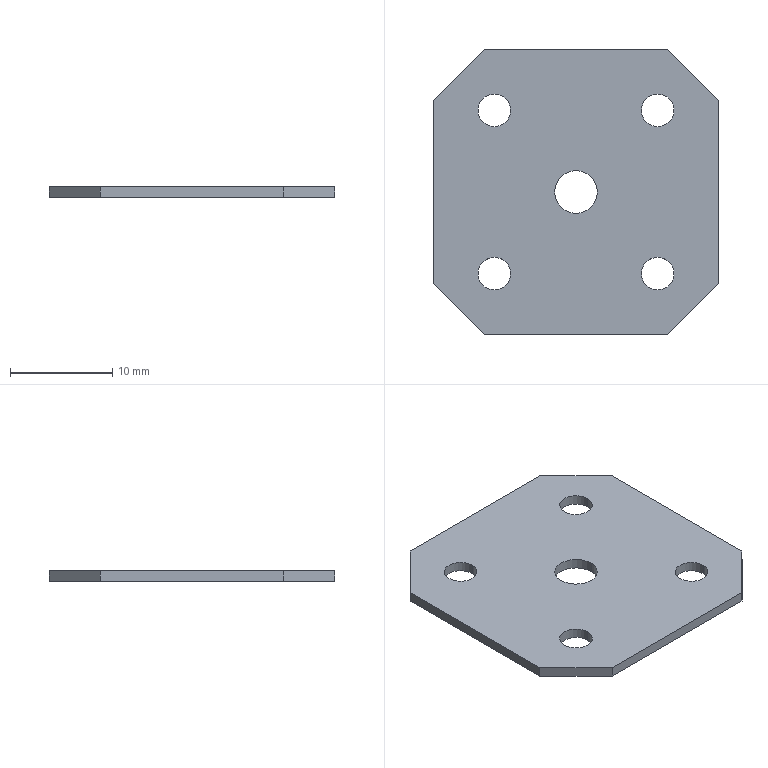Part | SolidWorks | features BaseBody 1 | 1 solid | 20 faces | box 28 x 28 x 1 mm | volume 688.173 mm3 | cylinder 10 | plane 10 | commonest cylinder face diameters 3.2 x8 4.17 x2
STEP:
#1=CARTESIAN_POINT('',(-2.085,0.,1.));
#2=VERTEX_POINT('',#1);
#3=CARTESIAN_POINT('',(2.085,0.,1.));
#4=VERTEX_POINT('',#3);
#5=CARTESIAN_POINT('',(0.,0.,1.));
#6=DIRECTION('',(0.,0.,1.));
#7=DIRECTION('',(-1.,0.,0.));
#8=AXIS2_PLACEMENT_3D('',#5,#6,#7);
#9=CIRCLE('',#8,2.085);
#10=EDGE_CURVE('',#2,#4,#9,.T.);
#11=ORIENTED_EDGE('',*,*,#10,.T.);
#12=CARTESIAN_POINT('',(2.085,0.,0.));
#13=VERTEX_POINT('',#12);
#14=CARTESIAN_POINT('',(2.085,0.,1.));
#15=DIRECTION('',(0.,0.,-1.));
#16=VECTOR('',#15,1000.);
#17=LINE('',#14,#16);
#18=EDGE_CURVE('',#4,#13,#17,.T.);
#19=ORIENTED_EDGE('',*,*,#18,.T.);
#20=CARTESIAN_POINT('',(-2.085,0.,0.));
#21=VERTEX_POINT('',#20);
#22=CARTESIAN_POINT('',(0.,0.,0.));
#23=DIRECTION('',(0.,0.,-1.));
#24=DIRECTION('',(-1.,0.,0.));
#25=AXIS2_PLACEMENT_3D('',#22,#23,#24);
#26=CIRCLE('',#25,2.085);
#27=EDGE_CURVE('',#13,#21,#26,.T.);
#28=ORIENTED_EDGE('',*,*,#27,.T.);
#29=CARTESIAN_POINT('',(-2.085,0.,1.));
#30=DIRECTION('',(0.,0.,-1.));
#31=VECTOR('',#30,1000.);
#32=LINE('',#29,#31);
#33=EDGE_CURVE('',#2,#21,#32,.T.);
#34=ORIENTED_EDGE('',*,*,#33,.F.);
#35=EDGE_LOOP('',(#11,#19,#28,#34));
#36=FACE_OUTER_BOUND('',#35,.T.);
#37=CARTESIAN_POINT('',(0.,0.,1.));
#38=DIRECTION('',(0.,0.,-1.));
#39=DIRECTION('',(-1.,0.,0.));
#40=AXIS2_PLACEMENT_3D('',#37,#38,#39);
#41=CYLINDRICAL_SURFACE('',#40,2.085);
#42=ADVANCED_FACE('',(#36),#41,.F.);
#43=CARTESIAN_POINT('',(9.6,-8.,1.));
#44=VERTEX_POINT('',#43);
#45=CARTESIAN_POINT('',(6.4,-8.,1.));
#46=VERTEX_POINT('',#45);
#47=CARTESIAN_POINT('',(8.,-8.,1.));
#48=DIRECTION('',(0.,0.,-1.));
#49=DIRECTION('',(-1.,0.,0.));
#50=AXIS2_PLACEMENT_3D('',#47,#48,#49);
#51=CIRCLE('',#50,1.6);
#52=EDGE_CURVE('',#44,#46,#51,.T.);
#53=ORIENTED_EDGE('',*,*,#52,.F.);
#54=CARTESIAN_POINT('',(9.6,-8.,0.));
#55=VERTEX_POINT('',#54);
#56=CARTESIAN_POINT('',(9.6,-8.,1.));
#57=DIRECTION('',(0.,0.,-1.));
#58=VECTOR('',#57,1000.);
#59=LINE('',#56,#58);
#60=EDGE_CURVE('',#44,#55,#59,.T.);
#61=ORIENTED_EDGE('',*,*,#60,.T.);
#62=CARTESIAN_POINT('',(6.4,-8.,0.));
#63=VERTEX_POINT('',#62);
#64=CARTESIAN_POINT('',(8.,-8.,0.));
#65=DIRECTION('',(0.,0.,-1.));
#66=DIRECTION('',(-1.,0.,0.));
#67=AXIS2_PLACEMENT_3D('',#64,#65,#66);
#68=CIRCLE('',#67,1.6);
#69=EDGE_CURVE('',#55,#63,#68,.T.);
#70=ORIENTED_EDGE('',*,*,#69,.T.);
#71=CARTESIAN_POINT('',(6.4,-8.,1.));
#72=DIRECTION('',(0.,0.,-1.));
#73=VECTOR('',#72,1000.);
#74=LINE('',#71,#73);
#75=EDGE_CURVE('',#46,#63,#74,.T.);
#76=ORIENTED_EDGE('',*,*,#75,.F.);
#77=EDGE_LOOP('',(#53,#61,#70,#76));
#78=FACE_OUTER_BOUND('',#77,.T.);
#79=CARTESIAN_POINT('',(8.,-8.,1.));
#80=DIRECTION('',(0.,0.,-1.));
#81=DIRECTION('',(-1.,0.,0.));
#82=AXIS2_PLACEMENT_3D('',#79,#80,#81);
#83=CYLINDRICAL_SURFACE('',#82,1.6);
#84=ADVANCED_FACE('',(#78),#83,.F.);
#85=CARTESIAN_POINT('',(-6.4,8.,1.));
#86=VERTEX_POINT('',#85);
#87=CARTESIAN_POINT('',(-9.6,8.,1.));
#88=VERTEX_POINT('',#87);
#89=CARTESIAN_POINT('',(-8.,8.,1.));
#90=DIRECTION('',(0.,0.,-1.));
#91=DIRECTION('',(-1.,0.,0.));
#92=AXIS2_PLACEMENT_3D('',#89,#90,#91);
#93=CIRCLE('',#92,1.6);
#94=EDGE_CURVE('',#86,#88,#93,.T.);
#95=ORIENTED_EDGE('',*,*,#94,.F.);
#96=CARTESIAN_POINT('',(-6.4,8.,0.));
#97=VERTEX_POINT('',#96);
#98=CARTESIAN_POINT('',(-6.4,8.,1.));
#99=DIRECTION('',(0.,0.,-1.));
#100=VECTOR('',#99,1000.);
#101=LINE('',#98,#100);
#102=EDGE_CURVE('',#86,#97,#101,.T.);
#103=ORIENTED_EDGE('',*,*,#102,.T.);
#104=CARTESIAN_POINT('',(-9.6,8.,0.));
#105=VERTEX_POINT('',#104);
#106=CARTESIAN_POINT('',(-8.,8.,0.));
#107=DIRECTION('',(0.,0.,-1.));
#108=DIRECTION('',(-1.,0.,0.));
#109=AXIS2_PLACEMENT_3D('',#106,#107,#108);
#110=CIRCLE('',#109,1.6);
#111=EDGE_CURVE('',#97,#105,#110,.T.);
#112=ORIENTED_EDGE('',*,*,#111,.T.);
#113=CARTESIAN_POINT('',(-9.6,8.,1.));
#114=DIRECTION('',(0.,0.,-1.));
#115=VECTOR('',#114,1000.);
#116=LINE('',#113,#115);
#117=EDGE_CURVE('',#88,#105,#116,.T.);
#118=ORIENTED_EDGE('',*,*,#117,.F.);
#119=EDGE_LOOP('',(#95,#103,#112,#118));
#120=FACE_OUTER_BOUND('',#119,.T.);
#121=CARTESIAN_POINT('',(-8.,8.,1.));
#122=DIRECTION('',(0.,0.,-1.));
#123=DIRECTION('',(-1.,0.,0.));
#124=AXIS2_PLACEMENT_3D('',#121,#122,#123);
#125=CYLINDRICAL_SURFACE('',#124,1.6);
#126=ADVANCED_FACE('',(#120),#125,.F.);
#127=CARTESIAN_POINT('',(9.6,8.,1.));
#128=VERTEX_POINT('',#127);
#129=CARTESIAN_POINT('',(6.4,8.,1.));
#130=VERTEX_POINT('',#129);
#131=CARTESIAN_POINT('',(8.,8.,1.));
#132=DIRECTION('',(0.,0.,-1.));
#133=DIRECTION('',(-1.,0.,0.));
#134=AXIS2_PLACEMENT_3D('',#131,#132,#133);
#135=CIRCLE('',#134,1.6);
#136=EDGE_CURVE('',#128,#130,#135,.T.);
#137=ORIENTED_EDGE('',*,*,#136,.F.);
#138=CARTESIAN_POINT('',(9.6,8.,0.));
#139=VERTEX_POINT('',#138);
#140=CARTESIAN_POINT('',(9.6,8.,1.));
#141=DIRECTION('',(0.,0.,-1.));
#142=VECTOR('',#141,1000.);
#143=LINE('',#140,#142);
#144=EDGE_CURVE('',#128,#139,#143,.T.);
#145=ORIENTED_EDGE('',*,*,#144,.T.);
#146=CARTESIAN_POINT('',(6.4,8.,0.));
#147=VERTEX_POINT('',#146);
#148=CARTESIAN_POINT('',(8.,8.,0.));
#149=DIRECTION('',(0.,0.,-1.));
#150=DIRECTION('',(-1.,0.,0.));
#151=AXIS2_PLACEMENT_3D('',#148,#149,#150);
#152=CIRCLE('',#151,1.6);
#153=EDGE_CURVE('',#139,#147,#152,.T.);
#154=ORIENTED_EDGE('',*,*,#153,.T.);
#155=CARTESIAN_POINT('',(6.4,8.,1.));
#156=DIRECTION('',(0.,0.,-1.));
#157=VECTOR('',#156,1000.);
#158=LINE('',#155,#157);
#159=EDGE_CURVE('',#130,#147,#158,.T.);
#160=ORIENTED_EDGE('',*,*,#159,.F.);
#161=EDGE_LOOP('',(#137,#145,#154,#160));
#162=FACE_OUTER_BOUND('',#161,.T.);
#163=CARTESIAN_POINT('',(8.,8.,1.));
#164=DIRECTION('',(0.,0.,-1.));
#165=DIRECTION('',(-1.,0.,0.));
#166=AXIS2_PLACEMENT_3D('',#163,#164,#165);
#167=CYLINDRICAL_SURFACE('',#166,1.6);
#168=ADVANCED_FACE('',(#162),#167,.F.);
#169=CARTESIAN_POINT('',(-6.4,-8.,1.));
#170=VERTEX_POINT('',#169);
#171=CARTESIAN_POINT('',(-9.6,-8.,1.));
#172=VERTEX_POINT('',#171);
#173=CARTESIAN_POINT('',(-8.,-8.,1.));
#174=DIRECTION('',(0.,0.,-1.));
#175=DIRECTION('',(-1.,0.,0.));
#176=AXIS2_PLACEMENT_3D('',#173,#174,#175);
#177=CIRCLE('',#176,1.6);
#178=EDGE_CURVE('',#170,#172,#177,.T.);
#179=ORIENTED_EDGE('',*,*,#178,.F.);
#180=CARTESIAN_POINT('',(-6.4,-8.,0.));
#181=VERTEX_POINT('',#180);
#182=CARTESIAN_POINT('',(-6.4,-8.,1.));
#183=DIRECTION('',(0.,0.,-1.));
#184=VECTOR('',#183,1000.);
#185=LINE('',#182,#184);
#186=EDGE_CURVE('',#170,#181,#185,.T.);
#187=ORIENTED_EDGE('',*,*,#186,.T.);
#188=CARTESIAN_POINT('',(-9.6,-8.,0.));
#189=VERTEX_POINT('',#188);
#190=CARTESIAN_POINT('',(-8.,-8.,0.));
#191=DIRECTION('',(0.,0.,-1.));
#192=DIRECTION('',(-1.,0.,0.));
#193=AXIS2_PLACEMENT_3D('',#190,#191,#192);
#194=CIRCLE('',#193,1.6);
#195=EDGE_CURVE('',#181,#189,#194,.T.);
#196=ORIENTED_EDGE('',*,*,#195,.T.);
#197=CARTESIAN_POINT('',(-9.6,-8.,1.));
#198=DIRECTION('',(0.,0.,-1.));
#199=VECTOR('',#198,1000.);
#200=LINE('',#197,#199);
#201=EDGE_CURVE('',#172,#189,#200,.T.);
#202=ORIENTED_EDGE('',*,*,#201,.F.);
#203=EDGE_LOOP('',(#179,#187,#196,#202));
#204=FACE_OUTER_BOUND('',#203,.T.);
#205=CARTESIAN_POINT('',(-8.,-8.,1.));
#206=DIRECTION('',(0.,0.,-1.));
#207=DIRECTION('',(-1.,0.,0.));
#208=AXIS2_PLACEMENT_3D('',#205,#206,#207);
#209=CYLINDRICAL_SURFACE('',#208,1.6);
#210=ADVANCED_FACE('',(#204),#209,.F.);
#211=ORIENTED_EDGE('',*,*,#18,.F.);
#212=CARTESIAN_POINT('',(0.,0.,1.));
#213=DIRECTION('',(0.,0.,1.));
#214=DIRECTION('',(-1.,0.,0.));
#215=AXIS2_PLACEMENT_3D('',#212,#213,#214);
#216=CIRCLE('',#215,2.085);
#217=EDGE_CURVE('',#4,#2,#216,.T.);
#218=ORIENTED_EDGE('',*,*,#217,.T.);
#219=ORIENTED_EDGE('',*,*,#33,.T.);
#220=CARTESIAN_POINT('',(0.,0.,0.));
#221=DIRECTION('',(0.,0.,-1.));
#222=DIRECTION('',(-1.,0.,0.));
#223=AXIS2_PLACEMENT_3D('',#220,#221,#222);
#224=CIRCLE('',#223,2.085);
#225=EDGE_CURVE('',#21,#13,#224,.T.);
#226=ORIENTED_EDGE('',*,*,#225,.T.);
#227=EDGE_LOOP('',(#211,#218,#219,#226));
#228=FACE_OUTER_BOUND('',#227,.T.);
#229=CARTESIAN_POINT('',(0.,0.,1.));
#230=DIRECTION('',(0.,0.,-1.));
#231=DIRECTION('',(-1.,0.,0.));
#232=AXIS2_PLACEMENT_3D('',#229,#230,#231);
#233=CYLINDRICAL_SURFACE('',#232,2.085);
#234=ADVANCED_FACE('',(#228),#233,.F.);
#235=ORIENTED_EDGE('',*,*,#225,.F.);
#236=ORIENTED_EDGE('',*,*,#27,.F.);
#237=EDGE_LOOP('',(#235,#236));
#238=FACE_BOUND('',#237,.T.);
#239=CARTESIAN_POINT('',(8.,-8.,0.));
#240=DIRECTION('',(0.,0.,-1.));
#241=DIRECTION('',(-1.,0.,0.));
#242=AXIS2_PLACEMENT_3D('',#239,#240,#241);
#243=CIRCLE('',#242,1.6);
#244=EDGE_CURVE('',#63,#55,#243,.T.);
#245=ORIENTED_EDGE('',*,*,#244,.F.);
#246=ORIENTED_EDGE('',*,*,#69,.F.);
#247=EDGE_LOOP('',(#245,#246));
#248=FACE_BOUND('',#247,.T.);
#249=CARTESIAN_POINT('',(-8.,8.,0.));
#250=DIRECTION('',(0.,0.,-1.));
#251=DIRECTION('',(-1.,0.,0.));
#252=AXIS2_PLACEMENT_3D('',#249,#250,#251);
#253=CIRCLE('',#252,1.6);
#254=EDGE_CURVE('',#105,#97,#253,.T.);
#255=ORIENTED_EDGE('',*,*,#254,.F.);
#256=ORIENTED_EDGE('',*,*,#111,.F.);
#257=EDGE_LOOP('',(#255,#256));
#258=FACE_BOUND('',#257,.T.);
#259=CARTESIAN_POINT('',(8.,8.,0.));
#260=DIRECTION('',(0.,0.,-1.));
#261=DIRECTION('',(-1.,0.,0.));
#262=AXIS2_PLACEMENT_3D('',#259,#260,#261);
#263=CIRCLE('',#262,1.6);
#264=EDGE_CURVE('',#147,#139,#263,.T.);
#265=ORIENTED_EDGE('',*,*,#264,.F.);
#266=ORIENTED_EDGE('',*,*,#153,.F.);
#267=EDGE_LOOP('',(#265,#266));
#268=FACE_BOUND('',#267,.T.);
#269=CARTESIAN_POINT('',(-8.,-8.,0.));
#270=DIRECTION('',(0.,0.,-1.));
#271=DIRECTION('',(-1.,0.,0.));
#272=AXIS2_PLACEMENT_3D('',#269,#270,#271);
#273=CIRCLE('',#272,1.6);
#274=EDGE_CURVE('',#189,#181,#273,.T.);
#275=ORIENTED_EDGE('',*,*,#274,.F.);
#276=ORIENTED_EDGE('',*,*,#195,.F.);
#277=EDGE_LOOP('',(#275,#276));
#278=FACE_BOUND('',#277,.T.);
#279=CARTESIAN_POINT('',(14.,9.,0.));
#280=VERTEX_POINT('',#279);
#281=CARTESIAN_POINT('',(9.,14.,0.));
#282=VERTEX_POINT('',#281);
#283=CARTESIAN_POINT('',(9.,14.,0.));
#284=DIRECTION('',(-0.7071,0.7071,0.));
#285=VECTOR('',#284,1000.);
#286=LINE('',#283,#285);
#287=EDGE_CURVE('',#280,#282,#286,.T.);
#288=ORIENTED_EDGE('',*,*,#287,.F.);
#289=CARTESIAN_POINT('',(14.,-9.,0.));
#290=VERTEX_POINT('',#289);
#291=CARTESIAN_POINT('',(14.,0.,0.));
#292=DIRECTION('',(0.,1.,0.));
#293=VECTOR('',#292,1000.);
#294=LINE('',#291,#293);
#295=EDGE_CURVE('',#290,#280,#294,.T.);
#296=ORIENTED_EDGE('',*,*,#295,.F.);
#297=CARTESIAN_POINT('',(9.,-14.,0.));
#298=VERTEX_POINT('',#297);
#299=CARTESIAN_POINT('',(14.,-9.,0.));
#300=DIRECTION('',(0.7071,0.7071,0.));
#301=VECTOR('',#300,1000.);
#302=LINE('',#299,#301);
#303=EDGE_CURVE('',#298,#290,#302,.T.);
#304=ORIENTED_EDGE('',*,*,#303,.F.);
#305=CARTESIAN_POINT('',(-9.,-14.,0.));
#306=VERTEX_POINT('',#305);
#307=CARTESIAN_POINT('',(0.,-14.,0.));
#308=DIRECTION('',(1.,0.,0.));
#309=VECTOR('',#308,1000.);
#310=LINE('',#307,#309);
#311=EDGE_CURVE('',#306,#298,#310,.T.);
#312=ORIENTED_EDGE('',*,*,#311,.F.);
#313=CARTESIAN_POINT('',(-14.,-9.,0.));
#314=VERTEX_POINT('',#313);
#315=CARTESIAN_POINT('',(-9.,-14.,0.));
#316=DIRECTION('',(0.7071,-0.7071,0.));
#317=VECTOR('',#316,1000.);
#318=LINE('',#315,#317);
#319=EDGE_CURVE('',#314,#306,#318,.T.);
#320=ORIENTED_EDGE('',*,*,#319,.F.);
#321=CARTESIAN_POINT('',(-14.,9.,0.));
#322=VERTEX_POINT('',#321);
#323=CARTESIAN_POINT('',(-14.,0.,0.));
#324=DIRECTION('',(0.,-1.,0.));
#325=VECTOR('',#324,1000.);
#326=LINE('',#323,#325);
#327=EDGE_CURVE('',#322,#314,#326,.T.);
#328=ORIENTED_EDGE('',*,*,#327,.F.);
#329=CARTESIAN_POINT('',(-9.,14.,0.));
#330=VERTEX_POINT('',#329);
#331=CARTESIAN_POINT('',(-14.,9.,0.));
#332=DIRECTION('',(-0.7071,-0.7071,0.));
#333=VECTOR('',#332,1000.);
#334=LINE('',#331,#333);
#335=EDGE_CURVE('',#330,#322,#334,.T.);
#336=ORIENTED_EDGE('',*,*,#335,.F.);
#337=CARTESIAN_POINT('',(0.,14.,0.));
#338=DIRECTION('',(-1.,0.,0.));
#339=VECTOR('',#338,1000.);
#340=LINE('',#337,#339);
#341=EDGE_CURVE('',#282,#330,#340,.T.);
#342=ORIENTED_EDGE('',*,*,#341,.F.);
#343=EDGE_LOOP('',(#288,#296,#304,#312,#320,#328,#336,#342));
#344=FACE_OUTER_BOUND('',#343,.T.);
#345=CARTESIAN_POINT('',(-14.,-14.,0.));
#346=DIRECTION('',(0.,0.,1.));
#347=DIRECTION('',(1.,0.,0.));
#348=AXIS2_PLACEMENT_3D('',#345,#346,#347);
#349=PLANE('',#348);
#350=ADVANCED_FACE('',(#238,#248,#258,#268,#278,#344),#349,.F.);
#351=ORIENTED_EDGE('',*,*,#10,.F.);
#352=ORIENTED_EDGE('',*,*,#217,.F.);
#353=EDGE_LOOP('',(#351,#352));
#354=FACE_BOUND('',#353,.T.);
#355=CARTESIAN_POINT('',(8.,-8.,1.));
#356=DIRECTION('',(0.,0.,-1.));
#357=DIRECTION('',(-1.,0.,0.));
#358=AXIS2_PLACEMENT_3D('',#355,#356,#357);
#359=CIRCLE('',#358,1.6);
#360=EDGE_CURVE('',#46,#44,#359,.T.);
#361=ORIENTED_EDGE('',*,*,#360,.T.);
#362=ORIENTED_EDGE('',*,*,#52,.T.);
#363=EDGE_LOOP('',(#361,#362));
#364=FACE_BOUND('',#363,.T.);
#365=CARTESIAN_POINT('',(-8.,8.,1.));
#366=DIRECTION('',(0.,0.,-1.));
#367=DIRECTION('',(-1.,0.,0.));
#368=AXIS2_PLACEMENT_3D('',#365,#366,#367);
#369=CIRCLE('',#368,1.6);
#370=EDGE_CURVE('',#88,#86,#369,.T.);
#371=ORIENTED_EDGE('',*,*,#370,.T.);
#372=ORIENTED_EDGE('',*,*,#94,.T.);
#373=EDGE_LOOP('',(#371,#372));
#374=FACE_BOUND('',#373,.T.);
#375=CARTESIAN_POINT('',(8.,8.,1.));
#376=DIRECTION('',(0.,0.,-1.));
#377=DIRECTION('',(-1.,0.,0.));
#378=AXIS2_PLACEMENT_3D('',#375,#376,#377);
#379=CIRCLE('',#378,1.6);
#380=EDGE_CURVE('',#130,#128,#379,.T.);
#381=ORIENTED_EDGE('',*,*,#380,.T.);
#382=ORIENTED_EDGE('',*,*,#136,.T.);
#383=EDGE_LOOP('',(#381,#382));
#384=FACE_BOUND('',#383,.T.);
#385=CARTESIAN_POINT('',(-8.,-8.,1.));
#386=DIRECTION('',(0.,0.,-1.));
#387=DIRECTION('',(-1.,0.,0.));
#388=AXIS2_PLACEMENT_3D('',#385,#386,#387);
#389=CIRCLE('',#388,1.6);
#390=EDGE_CURVE('',#172,#170,#389,.T.);
#391=ORIENTED_EDGE('',*,*,#390,.T.);
#392=ORIENTED_EDGE('',*,*,#178,.T.);
#393=EDGE_LOOP('',(#391,#392));
#394=FACE_BOUND('',#393,.T.);
#395=CARTESIAN_POINT('',(14.,-9.,1.));
#396=VERTEX_POINT('',#395);
#397=CARTESIAN_POINT('',(14.,9.,1.));
#398=VERTEX_POINT('',#397);
#399=CARTESIAN_POINT('',(14.,0.,1.));
#400=DIRECTION('',(0.,1.,0.));
#401=VECTOR('',#400,1000.);
#402=LINE('',#399,#401);
#403=EDGE_CURVE('',#396,#398,#402,.T.);
#404=ORIENTED_EDGE('',*,*,#403,.T.);
#405=CARTESIAN_POINT('',(9.,14.,1.));
#406=VERTEX_POINT('',#405);
#407=CARTESIAN_POINT('',(14.,9.,1.));
#408=DIRECTION('',(-0.7071,0.7071,0.));
#409=VECTOR('',#408,1000.);
#410=LINE('',#407,#409);
#411=EDGE_CURVE('',#398,#406,#410,.T.);
#412=ORIENTED_EDGE('',*,*,#411,.T.);
#413=CARTESIAN_POINT('',(-9.,14.,1.));
#414=VERTEX_POINT('',#413);
#415=CARTESIAN_POINT('',(0.,14.,1.));
#416=DIRECTION('',(-1.,0.,0.));
#417=VECTOR('',#416,1000.);
#418=LINE('',#415,#417);
#419=EDGE_CURVE('',#406,#414,#418,.T.);
#420=ORIENTED_EDGE('',*,*,#419,.T.);
#421=CARTESIAN_POINT('',(-14.,9.,1.));
#422=VERTEX_POINT('',#421);
#423=CARTESIAN_POINT('',(-9.,14.,1.));
#424=DIRECTION('',(-0.7071,-0.7071,0.));
#425=VECTOR('',#424,1000.);
#426=LINE('',#423,#425);
#427=EDGE_CURVE('',#414,#422,#426,.T.);
#428=ORIENTED_EDGE('',*,*,#427,.T.);
#429=CARTESIAN_POINT('',(-14.,-9.,1.));
#430=VERTEX_POINT('',#429);
#431=CARTESIAN_POINT('',(-14.,0.,1.));
#432=DIRECTION('',(0.,-1.,0.));
#433=VECTOR('',#432,1000.);
#434=LINE('',#431,#433);
#435=EDGE_CURVE('',#422,#430,#434,.T.);
#436=ORIENTED_EDGE('',*,*,#435,.T.);
#437=CARTESIAN_POINT('',(-9.,-14.,1.));
#438=VERTEX_POINT('',#437);
#439=CARTESIAN_POINT('',(-14.,-9.,1.));
#440=DIRECTION('',(0.7071,-0.7071,0.));
#441=VECTOR('',#440,1000.);
#442=LINE('',#439,#441);
#443=EDGE_CURVE('',#430,#438,#442,.T.);
#444=ORIENTED_EDGE('',*,*,#443,.T.);
#445=CARTESIAN_POINT('',(9.,-14.,1.));
#446=VERTEX_POINT('',#445);
#447=CARTESIAN_POINT('',(0.,-14.,1.));
#448=DIRECTION('',(1.,0.,0.));
#449=VECTOR('',#448,1000.);
#450=LINE('',#447,#449);
#451=EDGE_CURVE('',#438,#446,#450,.T.);
#452=ORIENTED_EDGE('',*,*,#451,.T.);
#453=CARTESIAN_POINT('',(9.,-14.,1.));
#454=DIRECTION('',(0.7071,0.7071,0.));
#455=VECTOR('',#454,1000.);
#456=LINE('',#453,#455);
#457=EDGE_CURVE('',#446,#396,#456,.T.);
#458=ORIENTED_EDGE('',*,*,#457,.T.);
#459=EDGE_LOOP('',(#404,#412,#420,#428,#436,#444,#452,#458));
#460=FACE_OUTER_BOUND('',#459,.T.);
#461=CARTESIAN_POINT('',(-14.,-14.,1.));
#462=DIRECTION('',(0.,0.,1.));
#463=DIRECTION('',(1.,0.,0.));
#464=AXIS2_PLACEMENT_3D('',#461,#462,#463);
#465=PLANE('',#464);
#466=ADVANCED_FACE('',(#354,#364,#374,#384,#394,#460),#465,.T.);
#467=ORIENTED_EDGE('',*,*,#60,.F.);
#468=ORIENTED_EDGE('',*,*,#360,.F.);
#469=ORIENTED_EDGE('',*,*,#75,.T.);
#470=ORIENTED_EDGE('',*,*,#244,.T.);
#471=EDGE_LOOP('',(#467,#468,#469,#470));
#472=FACE_OUTER_BOUND('',#471,.T.);
#473=CARTESIAN_POINT('',(8.,-8.,1.));
#474=DIRECTION('',(0.,0.,-1.));
#475=DIRECTION('',(-1.,0.,0.));
#476=AXIS2_PLACEMENT_3D('',#473,#474,#475);
#477=CYLINDRICAL_SURFACE('',#476,1.6);
#478=ADVANCED_FACE('',(#472),#477,.F.);
#479=ORIENTED_EDGE('',*,*,#102,.F.);
#480=ORIENTED_EDGE('',*,*,#370,.F.);
#481=ORIENTED_EDGE('',*,*,#117,.T.);
#482=ORIENTED_EDGE('',*,*,#254,.T.);
#483=EDGE_LOOP('',(#479,#480,#481,#482));
#484=FACE_OUTER_BOUND('',#483,.T.);
#485=CARTESIAN_POINT('',(-8.,8.,1.));
#486=DIRECTION('',(0.,0.,-1.));
#487=DIRECTION('',(-1.,0.,0.));
#488=AXIS2_PLACEMENT_3D('',#485,#486,#487);
#489=CYLINDRICAL_SURFACE('',#488,1.6);
#490=ADVANCED_FACE('',(#484),#489,.F.);
#491=ORIENTED_EDGE('',*,*,#144,.F.);
#492=ORIENTED_EDGE('',*,*,#380,.F.);
#493=ORIENTED_EDGE('',*,*,#159,.T.);
#494=ORIENTED_EDGE('',*,*,#264,.T.);
#495=EDGE_LOOP('',(#491,#492,#493,#494));
#496=FACE_OUTER_BOUND('',#495,.T.);
#497=CARTESIAN_POINT('',(8.,8.,1.));
#498=DIRECTION('',(0.,0.,-1.));
#499=DIRECTION('',(-1.,0.,0.));
#500=AXIS2_PLACEMENT_3D('',#497,#498,#499);
#501=CYLINDRICAL_SURFACE('',#500,1.6);
#502=ADVANCED_FACE('',(#496),#501,.F.);
#503=ORIENTED_EDGE('',*,*,#186,.F.);
#504=ORIENTED_EDGE('',*,*,#390,.F.);
#505=ORIENTED_EDGE('',*,*,#201,.T.);
#506=ORIENTED_EDGE('',*,*,#274,.T.);
#507=EDGE_LOOP('',(#503,#504,#505,#506));
#508=FACE_OUTER_BOUND('',#507,.T.);
#509=CARTESIAN_POINT('',(-8.,-8.,1.));
#510=DIRECTION('',(0.,0.,-1.));
#511=DIRECTION('',(-1.,0.,0.));
#512=AXIS2_PLACEMENT_3D('',#509,#510,#511);
#513=CYLINDRICAL_SURFACE('',#512,1.6);
#514=ADVANCED_FACE('',(#508),#513,.F.);
#515=CARTESIAN_POINT('',(-9.,14.,0.5));
#516=DIRECTION('',(0.,0.,-1.));
#517=VECTOR('',#516,1000.);
#518=LINE('',#515,#517);
#519=EDGE_CURVE('',#414,#330,#518,.T.);
#520=ORIENTED_EDGE('',*,*,#519,.F.);
#521=ORIENTED_EDGE('',*,*,#419,.F.);
#522=CARTESIAN_POINT('',(9.,14.,0.5));
#523=DIRECTION('',(0.,0.,1.));
#524=VECTOR('',#523,1000.);
#525=LINE('',#522,#524);
#526=EDGE_CURVE('',#282,#406,#525,.T.);
#527=ORIENTED_EDGE('',*,*,#526,.F.);
#528=ORIENTED_EDGE('',*,*,#341,.T.);
#529=EDGE_LOOP('',(#520,#521,#527,#528));
#530=FACE_OUTER_BOUND('',#529,.T.);
#531=CARTESIAN_POINT('',(-9.,14.,1.));
#532=DIRECTION('',(0.,-1.,0.));
#533=DIRECTION('',(0.,0.,-1.));
#534=AXIS2_PLACEMENT_3D('',#531,#532,#533);
#535=PLANE('',#534);
#536=ADVANCED_FACE('',(#530),#535,.F.);
#537=ORIENTED_EDGE('',*,*,#526,.T.);
#538=ORIENTED_EDGE('',*,*,#411,.F.);
#539=CARTESIAN_POINT('',(14.,9.,0.5));
#540=DIRECTION('',(0.,0.,1.));
#541=VECTOR('',#540,1000.);
#542=LINE('',#539,#541);
#543=EDGE_CURVE('',#280,#398,#542,.T.);
#544=ORIENTED_EDGE('',*,*,#543,.F.);
#545=ORIENTED_EDGE('',*,*,#287,.T.);
#546=EDGE_LOOP('',(#537,#538,#544,#545));
#547=FACE_OUTER_BOUND('',#546,.T.);
#548=CARTESIAN_POINT('',(9.,14.,0.));
#549=DIRECTION('',(-0.7071,-0.7071,0.));
#550=DIRECTION('',(0.7071,-0.7071,0.));
#551=AXIS2_PLACEMENT_3D('',#548,#549,#550);
#552=PLANE('',#551);
#553=ADVANCED_FACE('',(#547),#552,.F.);
#554=ORIENTED_EDGE('',*,*,#543,.T.);
#555=ORIENTED_EDGE('',*,*,#403,.F.);
#556=CARTESIAN_POINT('',(14.,-9.,0.5));
#557=DIRECTION('',(0.,0.,1.));
#558=VECTOR('',#557,1000.);
#559=LINE('',#556,#558);
#560=EDGE_CURVE('',#290,#396,#559,.T.);
#561=ORIENTED_EDGE('',*,*,#560,.F.);
#562=ORIENTED_EDGE('',*,*,#295,.T.);
#563=EDGE_LOOP('',(#554,#555,#561,#562));
#564=FACE_OUTER_BOUND('',#563,.T.);
#565=CARTESIAN_POINT('',(14.,9.,0.));
#566=DIRECTION('',(-1.,0.,0.));
#567=DIRECTION('',(0.,-1.,0.));
#568=AXIS2_PLACEMENT_3D('',#565,#566,#567);
#569=PLANE('',#568);
#570=ADVANCED_FACE('',(#564),#569,.F.);
#571=ORIENTED_EDGE('',*,*,#560,.T.);
#572=ORIENTED_EDGE('',*,*,#457,.F.);
#573=CARTESIAN_POINT('',(9.,-14.,0.5));
#574=DIRECTION('',(0.,0.,1.));
#575=VECTOR('',#574,1000.);
#576=LINE('',#573,#575);
#577=EDGE_CURVE('',#298,#446,#576,.T.);
#578=ORIENTED_EDGE('',*,*,#577,.F.);
#579=ORIENTED_EDGE('',*,*,#303,.T.);
#580=EDGE_LOOP('',(#571,#572,#578,#579));
#581=FACE_OUTER_BOUND('',#580,.T.);
#582=CARTESIAN_POINT('',(14.,-9.,0.));
#583=DIRECTION('',(-0.7071,0.7071,0.));
#584=DIRECTION('',(-0.7071,-0.7071,0.));
#585=AXIS2_PLACEMENT_3D('',#582,#583,#584);
#586=PLANE('',#585);
#587=ADVANCED_FACE('',(#581),#586,.F.);
#588=ORIENTED_EDGE('',*,*,#577,.T.);
#589=ORIENTED_EDGE('',*,*,#451,.F.);
#590=CARTESIAN_POINT('',(-9.,-14.,0.5));
#591=DIRECTION('',(0.,0.,1.));
#592=VECTOR('',#591,1000.);
#593=LINE('',#590,#592);
#594=EDGE_CURVE('',#306,#438,#593,.T.);
#595=ORIENTED_EDGE('',*,*,#594,.F.);
#596=ORIENTED_EDGE('',*,*,#311,.T.);
#597=EDGE_LOOP('',(#588,#589,#595,#596));
#598=FACE_OUTER_BOUND('',#597,.T.);
#599=CARTESIAN_POINT('',(-9.,-14.,0.));
#600=DIRECTION('',(0.,1.,0.));
#601=DIRECTION('',(0.,0.,1.));
#602=AXIS2_PLACEMENT_3D('',#599,#600,#601);
#603=PLANE('',#602);
#604=ADVANCED_FACE('',(#598),#603,.F.);
#605=ORIENTED_EDGE('',*,*,#594,.T.);
#606=ORIENTED_EDGE('',*,*,#443,.F.);
#607=CARTESIAN_POINT('',(-14.,-9.,0.5));
#608=DIRECTION('',(0.,0.,1.));
#609=VECTOR('',#608,1000.);
#610=LINE('',#607,#609);
#611=EDGE_CURVE('',#314,#430,#610,.T.);
#612=ORIENTED_EDGE('',*,*,#611,.F.);
#613=ORIENTED_EDGE('',*,*,#319,.T.);
#614=EDGE_LOOP('',(#605,#606,#612,#613));
#615=FACE_OUTER_BOUND('',#614,.T.);
#616=CARTESIAN_POINT('',(-9.,-14.,0.));
#617=DIRECTION('',(0.7071,0.7071,0.));
#618=DIRECTION('',(-0.7071,0.7071,0.));
#619=AXIS2_PLACEMENT_3D('',#616,#617,#618);
#620=PLANE('',#619);
#621=ADVANCED_FACE('',(#615),#620,.F.);
#622=ORIENTED_EDGE('',*,*,#611,.T.);
#623=ORIENTED_EDGE('',*,*,#435,.F.);
#624=CARTESIAN_POINT('',(-14.,9.,0.5));
#625=DIRECTION('',(0.,0.,1.));
#626=VECTOR('',#625,1000.);
#627=LINE('',#624,#626);
#628=EDGE_CURVE('',#322,#422,#627,.T.);
#629=ORIENTED_EDGE('',*,*,#628,.F.);
#630=ORIENTED_EDGE('',*,*,#327,.T.);
#631=EDGE_LOOP('',(#622,#623,#629,#630));
#632=FACE_OUTER_BOUND('',#631,.T.);
#633=CARTESIAN_POINT('',(-14.,-9.,0.));
#634=DIRECTION('',(1.,0.,0.));
#635=DIRECTION('',(0.,1.,0.));
#636=AXIS2_PLACEMENT_3D('',#633,#634,#635);
#637=PLANE('',#636);
#638=ADVANCED_FACE('',(#632),#637,.F.);
#639=ORIENTED_EDGE('',*,*,#628,.T.);
#640=ORIENTED_EDGE('',*,*,#427,.F.);
#641=ORIENTED_EDGE('',*,*,#519,.T.);
#642=ORIENTED_EDGE('',*,*,#335,.T.);
#643=EDGE_LOOP('',(#639,#640,#641,#642));
#644=FACE_OUTER_BOUND('',#643,.T.);
#645=CARTESIAN_POINT('',(-14.,9.,0.));
#646=DIRECTION('',(0.7071,-0.7071,0.));
#647=DIRECTION('',(0.7071,0.7071,0.));
#648=AXIS2_PLACEMENT_3D('',#645,#646,#647);
#649=PLANE('',#648);
#650=ADVANCED_FACE('',(#644),#649,.F.);
#651=CLOSED_SHELL('',(#42,#84,#126,#168,#210,#234,#350,#466,#478,#490,#502,#514,#536,#553,#570,#587,#604,#621,#638,#650));
#652=MANIFOLD_SOLID_BREP('',#651);
#653=CARTESIAN_POINT('',(0.,0.,0.));
#654=DIRECTION('',(0.,0.,1.));
#655=DIRECTION('',(1.,0.,0.));
#656=AXIS2_PLACEMENT_3D('',#653,#654,#655);
#657=(LENGTH_UNIT()NAMED_UNIT(*)SI_UNIT(.MILLI.,.METRE.));
#658=UNCERTAINTY_MEASURE_WITH_UNIT(LENGTH_MEASURE(0.00001),#657,'','');
#659=(NAMED_UNIT(*)PLANE_ANGLE_UNIT()SI_UNIT($,.RADIAN.));
#660=(NAMED_UNIT(*)SI_UNIT($,.STERADIAN.)SOLID_ANGLE_UNIT());
#661=(GEOMETRIC_REPRESENTATION_CONTEXT(3)GLOBAL_UNCERTAINTY_ASSIGNED_CONTEXT((#658))GLOBAL_UNIT_ASSIGNED_CONTEXT((#657,#659,#660))REPRESENTATION_CONTEXT('',''));
#662=ADVANCED_BREP_SHAPE_REPRESENTATION('',(#652,#656),#661);